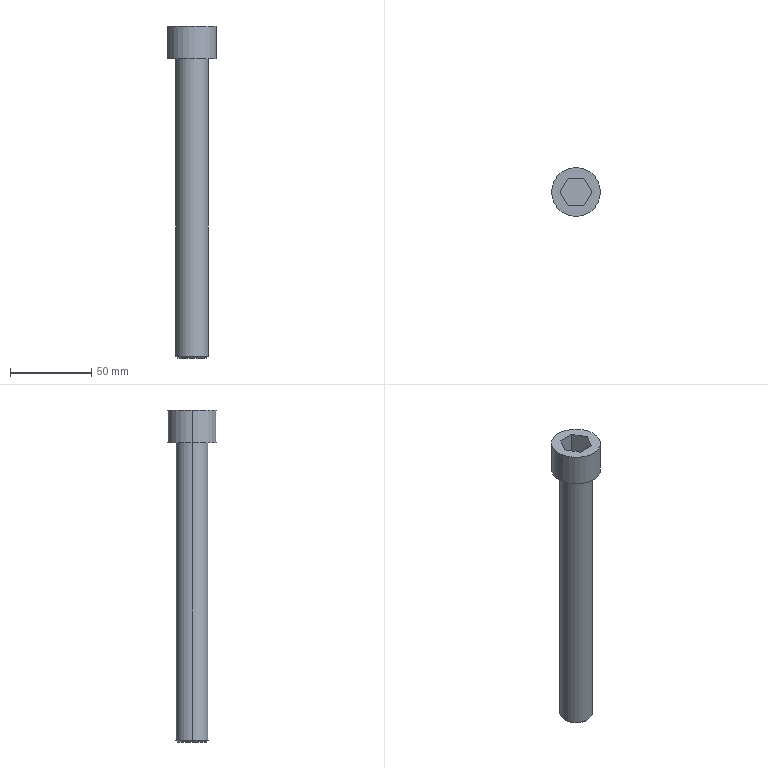Part | Creo | 1 solid | 16 faces | box 30 x 30 x 204 mm | volume 68607 mm3 | plane 10 | cylinder 4 | cone 2 | commonest cylinder face diameters 20 x2 30 x2
STEP:
#1=CARTESIAN_POINT('',(0.,0.,0.));
#2=DIRECTION('',(0.,0.,1.));
#3=DIRECTION('',(1.,0.,0.));
#4=AXIS2_PLACEMENT_3D('',#1,#2,#3);
#5=CARTESIAN_POINT('',(419.101,190.373,167.573));
#6=VERTEX_POINT('',#5);
#7=CARTESIAN_POINT('',(439.101,190.373,167.573));
#8=VERTEX_POINT('',#7);
#9=CARTESIAN_POINT('',(429.101,190.373,167.573));
#10=DIRECTION('',(0.,0.,-1.));
#11=DIRECTION('',(-1.,0.,0.));
#12=AXIS2_PLACEMENT_3D('',#9,#10,#11);
#13=CIRCLE('',#12,10.);
#14=EDGE_CURVE('',#6,#8,#13,.T.);
#15=ORIENTED_EDGE('',*,*,#14,.T.);
#16=CARTESIAN_POINT('',(439.101,190.373,350.559));
#17=VERTEX_POINT('',#16);
#18=CARTESIAN_POINT('',(439.101,190.373,350.559));
#19=DIRECTION('',(0.,0.,-1.));
#20=VECTOR('',#19,182.985);
#21=LINE('',#18,#20);
#22=EDGE_CURVE('',#17,#8,#21,.T.);
#23=ORIENTED_EDGE('',*,*,#22,.F.);
#24=CARTESIAN_POINT('',(419.101,190.373,350.559));
#25=VERTEX_POINT('',#24);
#26=CARTESIAN_POINT('',(429.101,190.373,350.559));
#27=DIRECTION('',(0.,0.,1.));
#28=DIRECTION('',(1.,0.,0.));
#29=AXIS2_PLACEMENT_3D('',#26,#27,#28);
#30=CIRCLE('',#29,10.);
#31=EDGE_CURVE('',#17,#25,#30,.T.);
#32=ORIENTED_EDGE('',*,*,#31,.T.);
#33=CARTESIAN_POINT('',(419.101,190.373,350.559));
#34=DIRECTION('',(0.,0.,-1.));
#35=VECTOR('',#34,182.985);
#36=LINE('',#33,#35);
#37=EDGE_CURVE('',#25,#6,#36,.T.);
#38=ORIENTED_EDGE('',*,*,#37,.T.);
#39=EDGE_LOOP('',(#15,#23,#32,#38));
#40=FACE_OUTER_BOUND('',#39,.F.);
#41=CARTESIAN_POINT('',(429.101,190.373,350.559));
#42=DIRECTION('',(0.,0.,-1.));
#43=DIRECTION('',(-1.,0.,0.));
#44=AXIS2_PLACEMENT_3D('',#41,#42,#43);
#45=CYLINDRICAL_SURFACE('',#44,10.);
#46=ADVANCED_FACE('',(#40),#45,.T.);
#47=CARTESIAN_POINT('',(420.116,190.373,166.559));
#48=VERTEX_POINT('',#47);
#49=CARTESIAN_POINT('',(438.086,190.373,166.559));
#50=VERTEX_POINT('',#49);
#51=CARTESIAN_POINT('',(429.101,190.373,166.559));
#52=DIRECTION('',(0.,0.,-1.));
#53=DIRECTION('',(-1.,0.,0.));
#54=AXIS2_PLACEMENT_3D('',#51,#52,#53);
#55=CIRCLE('',#54,8.985);
#56=EDGE_CURVE('',#48,#50,#55,.T.);
#57=ORIENTED_EDGE('',*,*,#56,.T.);
#58=CARTESIAN_POINT('',(438.086,190.373,166.559));
#59=DIRECTION('',(0.7071,0.,0.7071));
#60=VECTOR('',#59,1.435);
#61=LINE('',#58,#60);
#62=EDGE_CURVE('',#50,#8,#61,.T.);
#63=ORIENTED_EDGE('',*,*,#62,.T.);
#64=ORIENTED_EDGE('',*,*,#14,.F.);
#65=CARTESIAN_POINT('',(420.116,190.373,166.559));
#66=DIRECTION('',(-0.7071,0.,0.7071));
#67=VECTOR('',#66,1.435);
#68=LINE('',#65,#67);
#69=EDGE_CURVE('',#48,#6,#68,.T.);
#70=ORIENTED_EDGE('',*,*,#69,.F.);
#71=EDGE_LOOP('',(#57,#63,#64,#70));
#72=FACE_OUTER_BOUND('',#71,.F.);
#73=CARTESIAN_POINT('',(429.101,190.373,167.066));
#74=DIRECTION('',(0.,0.,1.));
#75=DIRECTION('',(1.,0.,0.));
#76=AXIS2_PLACEMENT_3D('',#73,#74,#75);
#77=CONICAL_SURFACE('',#76,9.493,45.);
#78=ADVANCED_FACE('',(#72),#77,.T.);
#79=CARTESIAN_POINT('',(429.101,190.373,166.559));
#80=DIRECTION('',(0.,0.,-1.));
#81=DIRECTION('',(1.,0.,0.));
#82=AXIS2_PLACEMENT_3D('',#79,#80,#81);
#83=CIRCLE('',#82,8.985);
#84=EDGE_CURVE('',#50,#48,#83,.T.);
#85=ORIENTED_EDGE('',*,*,#84,.F.);
#86=ORIENTED_EDGE('',*,*,#56,.F.);
#87=EDGE_LOOP('',(#85,#86));
#88=FACE_OUTER_BOUND('',#87,.F.);
#89=CARTESIAN_POINT('',(429.101,190.373,166.559));
#90=DIRECTION('',(0.,0.,1.));
#91=DIRECTION('',(1.,0.,0.));
#92=AXIS2_PLACEMENT_3D('',#89,#90,#91);
#93=PLANE('',#92);
#94=ADVANCED_FACE('',(#88),#93,.F.);
#95=ORIENTED_EDGE('',*,*,#84,.T.);
#96=ORIENTED_EDGE('',*,*,#69,.T.);
#97=CARTESIAN_POINT('',(429.101,190.373,167.573));
#98=DIRECTION('',(0.,0.,-1.));
#99=DIRECTION('',(1.,0.,0.));
#100=AXIS2_PLACEMENT_3D('',#97,#98,#99);
#101=CIRCLE('',#100,10.);
#102=EDGE_CURVE('',#8,#6,#101,.T.);
#103=ORIENTED_EDGE('',*,*,#102,.F.);
#104=ORIENTED_EDGE('',*,*,#62,.F.);
#105=EDGE_LOOP('',(#95,#96,#103,#104));
#106=FACE_OUTER_BOUND('',#105,.F.);
#107=CARTESIAN_POINT('',(429.101,190.373,167.066));
#108=DIRECTION('',(0.,0.,1.));
#109=DIRECTION('',(1.,0.,0.));
#110=AXIS2_PLACEMENT_3D('',#107,#108,#109);
#111=CONICAL_SURFACE('',#110,9.493,45.);
#112=ADVANCED_FACE('',(#106),#111,.T.);
#113=ORIENTED_EDGE('',*,*,#102,.T.);
#114=ORIENTED_EDGE('',*,*,#37,.F.);
#115=CARTESIAN_POINT('',(429.101,190.373,350.559));
#116=DIRECTION('',(0.,0.,1.));
#117=DIRECTION('',(-1.,0.,0.));
#118=AXIS2_PLACEMENT_3D('',#115,#116,#117);
#119=CIRCLE('',#118,10.);
#120=EDGE_CURVE('',#25,#17,#119,.T.);
#121=ORIENTED_EDGE('',*,*,#120,.T.);
#122=ORIENTED_EDGE('',*,*,#22,.T.);
#123=EDGE_LOOP('',(#113,#114,#121,#122));
#124=FACE_OUTER_BOUND('',#123,.F.);
#125=CARTESIAN_POINT('',(429.101,190.373,350.559));
#126=DIRECTION('',(0.,0.,-1.));
#127=DIRECTION('',(-1.,0.,0.));
#128=AXIS2_PLACEMENT_3D('',#125,#126,#127);
#129=CYLINDRICAL_SURFACE('',#128,10.);
#130=ADVANCED_FACE('',(#124),#129,.T.);
#131=CARTESIAN_POINT('',(444.101,190.373,350.559));
#132=VERTEX_POINT('',#131);
#133=CARTESIAN_POINT('',(414.101,190.373,350.559));
#134=VERTEX_POINT('',#133);
#135=CARTESIAN_POINT('',(429.101,190.373,350.559));
#136=DIRECTION('',(0.,0.,-1.));
#137=DIRECTION('',(1.,0.,0.));
#138=AXIS2_PLACEMENT_3D('',#135,#136,#137);
#139=CIRCLE('',#138,15.);
#140=EDGE_CURVE('',#132,#134,#139,.T.);
#141=ORIENTED_EDGE('',*,*,#140,.F.);
#142=CARTESIAN_POINT('',(429.101,190.373,350.559));
#143=DIRECTION('',(0.,0.,-1.));
#144=DIRECTION('',(-1.,0.,0.));
#145=AXIS2_PLACEMENT_3D('',#142,#143,#144);
#146=CIRCLE('',#145,15.);
#147=EDGE_CURVE('',#134,#132,#146,.T.);
#148=ORIENTED_EDGE('',*,*,#147,.F.);
#149=EDGE_LOOP('',(#141,#148));
#150=FACE_OUTER_BOUND('',#149,.F.);
#151=ORIENTED_EDGE('',*,*,#31,.F.);
#152=ORIENTED_EDGE('',*,*,#120,.F.);
#153=EDGE_LOOP('',(#151,#152));
#154=FACE_BOUND('',#153,.F.);
#155=CARTESIAN_POINT('',(429.101,190.373,350.559));
#156=DIRECTION('',(0.,0.,-1.));
#157=DIRECTION('',(-1.,0.,0.));
#158=AXIS2_PLACEMENT_3D('',#155,#156,#157);
#159=PLANE('',#158);
#160=ADVANCED_FACE('',(#150,#154),#159,.T.);
#161=CARTESIAN_POINT('',(414.101,190.373,370.559));
#162=VERTEX_POINT('',#161);
#163=CARTESIAN_POINT('',(444.101,190.373,370.559));
#164=VERTEX_POINT('',#163);
#165=CARTESIAN_POINT('',(429.101,190.373,370.559));
#166=DIRECTION('',(0.,0.,1.));
#167=DIRECTION('',(-1.,0.,0.));
#168=AXIS2_PLACEMENT_3D('',#165,#166,#167);
#169=CIRCLE('',#168,15.);
#170=EDGE_CURVE('',#162,#164,#169,.T.);
#171=ORIENTED_EDGE('',*,*,#170,.T.);
#172=CARTESIAN_POINT('',(444.101,190.373,350.559));
#173=DIRECTION('',(0.,0.,1.));
#174=VECTOR('',#173,20.);
#175=LINE('',#172,#174);
#176=EDGE_CURVE('',#132,#164,#175,.T.);
#177=ORIENTED_EDGE('',*,*,#176,.F.);
#178=ORIENTED_EDGE('',*,*,#140,.T.);
#179=CARTESIAN_POINT('',(414.101,190.373,350.559));
#180=DIRECTION('',(0.,0.,1.));
#181=VECTOR('',#180,20.);
#182=LINE('',#179,#181);
#183=EDGE_CURVE('',#134,#162,#182,.T.);
#184=ORIENTED_EDGE('',*,*,#183,.T.);
#185=EDGE_LOOP('',(#171,#177,#178,#184));
#186=FACE_OUTER_BOUND('',#185,.F.);
#187=CARTESIAN_POINT('',(429.101,190.373,350.559));
#188=DIRECTION('',(0.,0.,1.));
#189=DIRECTION('',(1.,0.,0.));
#190=AXIS2_PLACEMENT_3D('',#187,#188,#189);
#191=CYLINDRICAL_SURFACE('',#190,15.);
#192=ADVANCED_FACE('',(#186),#191,.T.);
#193=CARTESIAN_POINT('',(429.101,190.373,370.559));
#194=DIRECTION('',(0.,0.,1.));
#195=DIRECTION('',(1.,0.,0.));
#196=AXIS2_PLACEMENT_3D('',#193,#194,#195);
#197=CIRCLE('',#196,15.);
#198=EDGE_CURVE('',#164,#162,#197,.T.);
#199=ORIENTED_EDGE('',*,*,#198,.F.);
#200=ORIENTED_EDGE('',*,*,#170,.F.);
#201=EDGE_LOOP('',(#199,#200));
#202=FACE_OUTER_BOUND('',#201,.F.);
#203=CARTESIAN_POINT('',(434.008,181.873,370.559));
#204=VERTEX_POINT('',#203);
#205=CARTESIAN_POINT('',(424.193,181.873,370.559));
#206=VERTEX_POINT('',#205);
#207=CARTESIAN_POINT('',(434.008,181.873,370.559));
#208=DIRECTION('',(-1.,0.,0.));
#209=VECTOR('',#208,9.815);
#210=LINE('',#207,#209);
#211=EDGE_CURVE('',#204,#206,#210,.T.);
#212=ORIENTED_EDGE('',*,*,#211,.F.);
#213=CARTESIAN_POINT('',(438.916,190.373,370.559));
#214=VERTEX_POINT('',#213);
#215=CARTESIAN_POINT('',(438.916,190.373,370.559));
#216=DIRECTION('',(-0.5,-0.866,0.));
#217=VECTOR('',#216,9.815);
#218=LINE('',#215,#217);
#219=EDGE_CURVE('',#214,#204,#218,.T.);
#220=ORIENTED_EDGE('',*,*,#219,.F.);
#221=CARTESIAN_POINT('',(434.008,198.873,370.559));
#222=VERTEX_POINT('',#221);
#223=CARTESIAN_POINT('',(434.008,198.873,370.559));
#224=DIRECTION('',(0.5,-0.866,0.));
#225=VECTOR('',#224,9.815);
#226=LINE('',#223,#225);
#227=EDGE_CURVE('',#222,#214,#226,.T.);
#228=ORIENTED_EDGE('',*,*,#227,.F.);
#229=CARTESIAN_POINT('',(424.193,198.873,370.559));
#230=VERTEX_POINT('',#229);
#231=CARTESIAN_POINT('',(424.193,198.873,370.559));
#232=DIRECTION('',(1.,0.,0.));
#233=VECTOR('',#232,9.815);
#234=LINE('',#231,#233);
#235=EDGE_CURVE('',#230,#222,#234,.T.);
#236=ORIENTED_EDGE('',*,*,#235,.F.);
#237=CARTESIAN_POINT('',(419.286,190.373,370.559));
#238=VERTEX_POINT('',#237);
#239=CARTESIAN_POINT('',(419.286,190.373,370.559));
#240=DIRECTION('',(0.5,0.866,0.));
#241=VECTOR('',#240,9.815);
#242=LINE('',#239,#241);
#243=EDGE_CURVE('',#238,#230,#242,.T.);
#244=ORIENTED_EDGE('',*,*,#243,.F.);
#245=CARTESIAN_POINT('',(424.193,181.873,370.559));
#246=DIRECTION('',(-0.5,0.866,0.));
#247=VECTOR('',#246,9.815);
#248=LINE('',#245,#247);
#249=EDGE_CURVE('',#206,#238,#248,.T.);
#250=ORIENTED_EDGE('',*,*,#249,.F.);
#251=EDGE_LOOP('',(#212,#220,#228,#236,#244,#250));
#252=FACE_BOUND('',#251,.F.);
#253=CARTESIAN_POINT('',(429.101,190.373,370.559));
#254=DIRECTION('',(0.,0.,1.));
#255=DIRECTION('',(1.,0.,0.));
#256=AXIS2_PLACEMENT_3D('',#253,#254,#255);
#257=PLANE('',#256);
#258=ADVANCED_FACE('',(#202,#252),#257,.T.);
#259=ORIENTED_EDGE('',*,*,#211,.T.);
#260=CARTESIAN_POINT('',(424.193,181.873,357.359));
#261=VERTEX_POINT('',#260);
#262=CARTESIAN_POINT('',(424.193,181.873,370.559));
#263=DIRECTION('',(0.,0.,-1.));
#264=VECTOR('',#263,13.2);
#265=LINE('',#262,#264);
#266=EDGE_CURVE('',#206,#261,#265,.T.);
#267=ORIENTED_EDGE('',*,*,#266,.T.);
#268=CARTESIAN_POINT('',(434.008,181.873,357.359));
#269=VERTEX_POINT('',#268);
#270=CARTESIAN_POINT('',(434.008,181.873,357.359));
#271=DIRECTION('',(-1.,0.,0.));
#272=VECTOR('',#271,9.815);
#273=LINE('',#270,#272);
#274=EDGE_CURVE('',#269,#261,#273,.T.);
#275=ORIENTED_EDGE('',*,*,#274,.F.);
#276=CARTESIAN_POINT('',(434.008,181.873,370.559));
#277=DIRECTION('',(0.,0.,-1.));
#278=VECTOR('',#277,13.2);
#279=LINE('',#276,#278);
#280=EDGE_CURVE('',#204,#269,#279,.T.);
#281=ORIENTED_EDGE('',*,*,#280,.F.);
#282=EDGE_LOOP('',(#259,#267,#275,#281));
#283=FACE_OUTER_BOUND('',#282,.F.);
#284=CARTESIAN_POINT('',(424.193,181.873,357.359));
#285=DIRECTION('',(0.,-1.,0.));
#286=DIRECTION('',(0.,0.,-1.));
#287=AXIS2_PLACEMENT_3D('',#284,#285,#286);
#288=PLANE('',#287);
#289=ADVANCED_FACE('',(#283),#288,.F.);
#290=ORIENTED_EDGE('',*,*,#249,.T.);
#291=CARTESIAN_POINT('',(419.286,190.373,357.359));
#292=VERTEX_POINT('',#291);
#293=CARTESIAN_POINT('',(419.286,190.373,370.559));
#294=DIRECTION('',(0.,0.,-1.));
#295=VECTOR('',#294,13.2);
#296=LINE('',#293,#295);
#297=EDGE_CURVE('',#238,#292,#296,.T.);
#298=ORIENTED_EDGE('',*,*,#297,.T.);
#299=CARTESIAN_POINT('',(419.286,190.373,357.359));
#300=DIRECTION('',(0.5,-0.866,0.));
#301=VECTOR('',#300,9.815);
#302=LINE('',#299,#301);
#303=EDGE_CURVE('',#292,#261,#302,.T.);
#304=ORIENTED_EDGE('',*,*,#303,.T.);
#305=ORIENTED_EDGE('',*,*,#266,.F.);
#306=EDGE_LOOP('',(#290,#298,#304,#305));
#307=FACE_OUTER_BOUND('',#306,.F.);
#308=CARTESIAN_POINT('',(419.286,190.373,357.359));
#309=DIRECTION('',(-0.866,-0.5,0.));
#310=DIRECTION('',(0.5,-0.866,0.));
#311=AXIS2_PLACEMENT_3D('',#308,#309,#310);
#312=PLANE('',#311);
#313=ADVANCED_FACE('',(#307),#312,.F.);
#314=ORIENTED_EDGE('',*,*,#243,.T.);
#315=CARTESIAN_POINT('',(424.193,198.873,357.359));
#316=VERTEX_POINT('',#315);
#317=CARTESIAN_POINT('',(424.193,198.873,370.559));
#318=DIRECTION('',(0.,0.,-1.));
#319=VECTOR('',#318,13.2);
#320=LINE('',#317,#319);
#321=EDGE_CURVE('',#230,#316,#320,.T.);
#322=ORIENTED_EDGE('',*,*,#321,.T.);
#323=CARTESIAN_POINT('',(424.193,198.873,357.359));
#324=DIRECTION('',(-0.5,-0.866,0.));
#325=VECTOR('',#324,9.815);
#326=LINE('',#323,#325);
#327=EDGE_CURVE('',#316,#292,#326,.T.);
#328=ORIENTED_EDGE('',*,*,#327,.T.);
#329=ORIENTED_EDGE('',*,*,#297,.F.);
#330=EDGE_LOOP('',(#314,#322,#328,#329));
#331=FACE_OUTER_BOUND('',#330,.F.);
#332=CARTESIAN_POINT('',(424.193,198.873,357.359));
#333=DIRECTION('',(-0.866,0.5,0.));
#334=DIRECTION('',(-0.5,-0.866,0.));
#335=AXIS2_PLACEMENT_3D('',#332,#333,#334);
#336=PLANE('',#335);
#337=ADVANCED_FACE('',(#331),#336,.F.);
#338=ORIENTED_EDGE('',*,*,#235,.T.);
#339=CARTESIAN_POINT('',(434.008,198.873,357.359));
#340=VERTEX_POINT('',#339);
#341=CARTESIAN_POINT('',(434.008,198.873,370.559));
#342=DIRECTION('',(0.,0.,-1.));
#343=VECTOR('',#342,13.2);
#344=LINE('',#341,#343);
#345=EDGE_CURVE('',#222,#340,#344,.T.);
#346=ORIENTED_EDGE('',*,*,#345,.T.);
#347=CARTESIAN_POINT('',(424.193,198.873,357.359));
#348=DIRECTION('',(1.,0.,0.));
#349=VECTOR('',#348,9.815);
#350=LINE('',#347,#349);
#351=EDGE_CURVE('',#316,#340,#350,.T.);
#352=ORIENTED_EDGE('',*,*,#351,.F.);
#353=ORIENTED_EDGE('',*,*,#321,.F.);
#354=EDGE_LOOP('',(#338,#346,#352,#353));
#355=FACE_OUTER_BOUND('',#354,.F.);
#356=CARTESIAN_POINT('',(434.008,198.873,357.359));
#357=DIRECTION('',(0.,1.,0.));
#358=DIRECTION('',(0.,0.,1.));
#359=AXIS2_PLACEMENT_3D('',#356,#357,#358);
#360=PLANE('',#359);
#361=ADVANCED_FACE('',(#355),#360,.F.);
#362=ORIENTED_EDGE('',*,*,#227,.T.);
#363=CARTESIAN_POINT('',(438.916,190.373,357.359));
#364=VERTEX_POINT('',#363);
#365=CARTESIAN_POINT('',(438.916,190.373,370.559));
#366=DIRECTION('',(0.,0.,-1.));
#367=VECTOR('',#366,13.2);
#368=LINE('',#365,#367);
#369=EDGE_CURVE('',#214,#364,#368,.T.);
#370=ORIENTED_EDGE('',*,*,#369,.T.);
#371=CARTESIAN_POINT('',(438.916,190.373,357.359));
#372=DIRECTION('',(-0.5,0.866,0.));
#373=VECTOR('',#372,9.815);
#374=LINE('',#371,#373);
#375=EDGE_CURVE('',#364,#340,#374,.T.);
#376=ORIENTED_EDGE('',*,*,#375,.T.);
#377=ORIENTED_EDGE('',*,*,#345,.F.);
#378=EDGE_LOOP('',(#362,#370,#376,#377));
#379=FACE_OUTER_BOUND('',#378,.F.);
#380=CARTESIAN_POINT('',(438.916,190.373,357.359));
#381=DIRECTION('',(0.866,0.5,0.));
#382=DIRECTION('',(-0.5,0.866,0.));
#383=AXIS2_PLACEMENT_3D('',#380,#381,#382);
#384=PLANE('',#383);
#385=ADVANCED_FACE('',(#379),#384,.F.);
#386=ORIENTED_EDGE('',*,*,#219,.T.);
#387=ORIENTED_EDGE('',*,*,#280,.T.);
#388=CARTESIAN_POINT('',(434.008,181.873,357.359));
#389=DIRECTION('',(0.5,0.866,0.));
#390=VECTOR('',#389,9.815);
#391=LINE('',#388,#390);
#392=EDGE_CURVE('',#269,#364,#391,.T.);
#393=ORIENTED_EDGE('',*,*,#392,.T.);
#394=ORIENTED_EDGE('',*,*,#369,.F.);
#395=EDGE_LOOP('',(#386,#387,#393,#394));
#396=FACE_OUTER_BOUND('',#395,.F.);
#397=CARTESIAN_POINT('',(434.008,181.873,357.359));
#398=DIRECTION('',(0.866,-0.5,0.));
#399=DIRECTION('',(0.5,0.866,0.));
#400=AXIS2_PLACEMENT_3D('',#397,#398,#399);
#401=PLANE('',#400);
#402=ADVANCED_FACE('',(#396),#401,.F.);
#403=ORIENTED_EDGE('',*,*,#274,.T.);
#404=ORIENTED_EDGE('',*,*,#303,.F.);
#405=ORIENTED_EDGE('',*,*,#327,.F.);
#406=ORIENTED_EDGE('',*,*,#351,.T.);
#407=ORIENTED_EDGE('',*,*,#375,.F.);
#408=ORIENTED_EDGE('',*,*,#392,.F.);
#409=EDGE_LOOP('',(#403,#404,#405,#406,#407,#408));
#410=FACE_OUTER_BOUND('',#409,.F.);
#411=CARTESIAN_POINT('',(434.008,181.873,357.359));
#412=DIRECTION('',(0.,0.,1.));
#413=DIRECTION('',(1.,0.,0.));
#414=AXIS2_PLACEMENT_3D('',#411,#412,#413);
#415=PLANE('',#414);
#416=ADVANCED_FACE('',(#410),#415,.T.);
#417=ORIENTED_EDGE('',*,*,#198,.T.);
#418=ORIENTED_EDGE('',*,*,#183,.F.);
#419=ORIENTED_EDGE('',*,*,#147,.T.);
#420=ORIENTED_EDGE('',*,*,#176,.T.);
#421=EDGE_LOOP('',(#417,#418,#419,#420));
#422=FACE_OUTER_BOUND('',#421,.F.);
#423=CARTESIAN_POINT('',(429.101,190.373,350.559));
#424=DIRECTION('',(0.,0.,1.));
#425=DIRECTION('',(1.,0.,0.));
#426=AXIS2_PLACEMENT_3D('',#423,#424,#425);
#427=CYLINDRICAL_SURFACE('',#426,15.);
#428=ADVANCED_FACE('',(#422),#427,.T.);
#429=CLOSED_SHELL('',(#46,#78,#94,#112,#130,#160,#192,#258,#289,#313,#337,#361,#385,#402,#416,#428));
#430=MANIFOLD_SOLID_BREP('',#429);
#431=(LENGTH_UNIT()NAMED_UNIT(*)SI_UNIT(.MILLI.,.METRE.));
#432=UNCERTAINTY_MEASURE_WITH_UNIT(LENGTH_MEASURE(0.02084),#431,'','');
#433=(NAMED_UNIT(*)PLANE_ANGLE_UNIT()SI_UNIT($,.RADIAN.));
#434=PLANE_ANGLE_MEASURE_WITH_UNIT(PLANE_ANGLE_MEASURE(0.01745),#433);
#435=(CONVERSION_BASED_UNIT('DEGREE',#434)NAMED_UNIT(*)PLANE_ANGLE_UNIT());
#436=(NAMED_UNIT(*)SI_UNIT($,.STERADIAN.)SOLID_ANGLE_UNIT());
#437=(GEOMETRIC_REPRESENTATION_CONTEXT(3)GLOBAL_UNCERTAINTY_ASSIGNED_CONTEXT((#432))GLOBAL_UNIT_ASSIGNED_CONTEXT((#431,#435,#436))REPRESENTATION_CONTEXT('',''));
#438=ADVANCED_BREP_SHAPE_REPRESENTATION('',(#4,#430),#437);